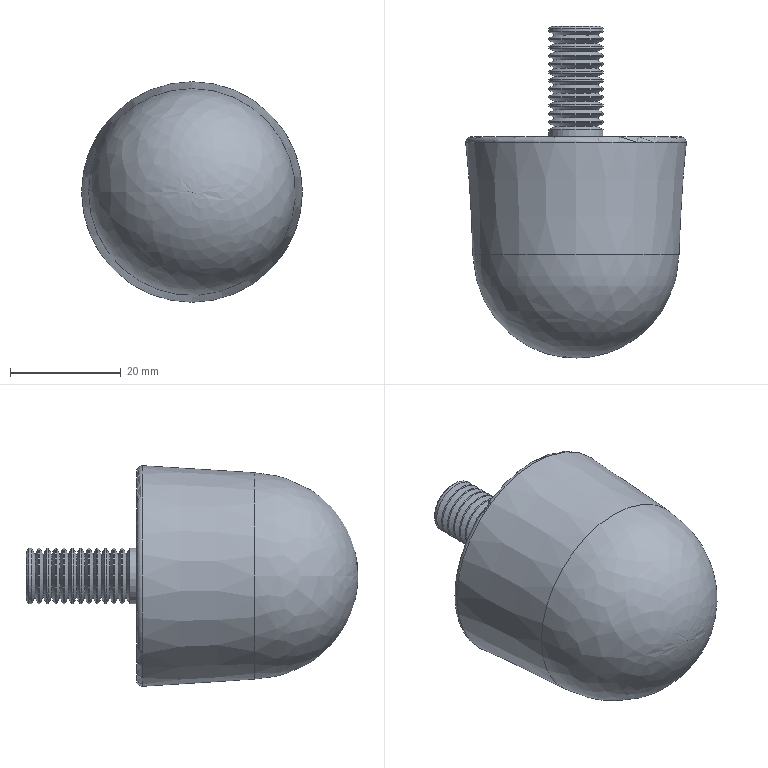Part | STEP file | 5091301W | 1 solid | 43 faces | box 39.871 x 60 x 39.871 mm | volume 39857 mm3 | cone 26 | cylinder 13 | plane 2 | torus 1 | spline 1 | commonest cylinder face diameters 10 x13